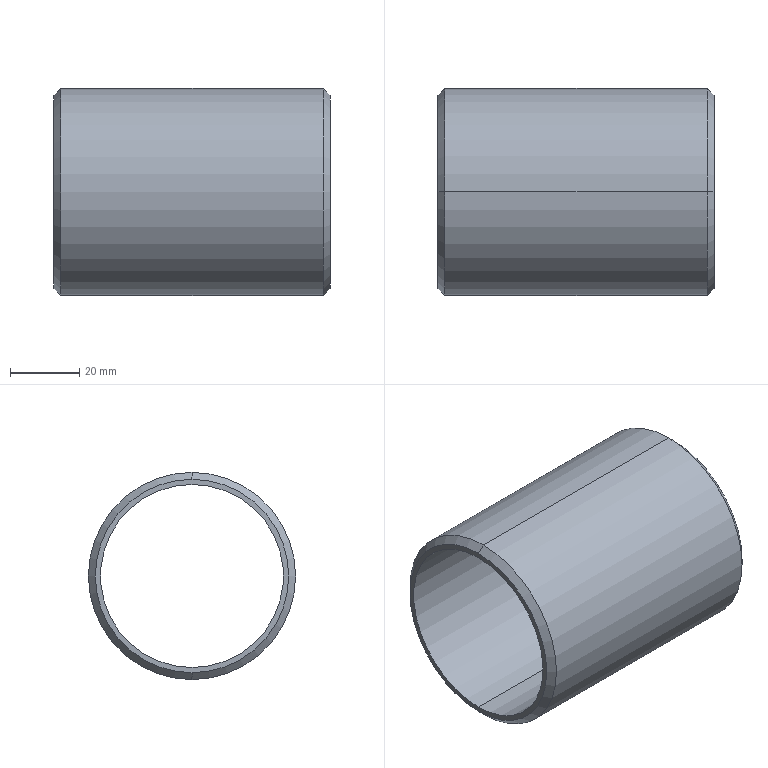Part | SolidWorks | features Chamfer 1, ExtruThin 1 | 1 solid | 10 faces | box 80 x 60 x 60 mm | volume 48963 mm3 | cone 4 | cylinder 4 | plane 2 | commonest cylinder face diameters 53 x2 60 x2
STEP:
#1=CARTESIAN_POINT('',(0.,0.,28.));
#2=VERTEX_POINT('',#1);
#3=CARTESIAN_POINT('',(0.,0.,-28.));
#4=VERTEX_POINT('',#3);
#5=CARTESIAN_POINT('',(0.,0.,0.));
#6=DIRECTION('',(-1.,0.,0.));
#7=DIRECTION('',(0.,0.,-1.));
#8=AXIS2_PLACEMENT_3D('',#5,#6,#7);
#9=CIRCLE('',#8,28.);
#10=EDGE_CURVE('',#2,#4,#9,.T.);
#11=ORIENTED_EDGE('',*,*,#10,.F.);
#12=CARTESIAN_POINT('',(2.,0.,30.));
#13=VERTEX_POINT('',#12);
#14=CARTESIAN_POINT('',(2.,0.,30.));
#15=DIRECTION('',(0.7071,0.,0.7071));
#16=VECTOR('',#15,1000.);
#17=LINE('',#14,#16);
#18=EDGE_CURVE('',#2,#13,#17,.T.);
#19=ORIENTED_EDGE('',*,*,#18,.T.);
#20=CARTESIAN_POINT('',(2.,0.,-30.));
#21=VERTEX_POINT('',#20);
#22=CARTESIAN_POINT('',(2.,0.,0.));
#23=DIRECTION('',(1.,0.,0.));
#24=DIRECTION('',(0.,0.,-1.));
#25=AXIS2_PLACEMENT_3D('',#22,#23,#24);
#26=CIRCLE('',#25,30.);
#27=EDGE_CURVE('',#21,#13,#26,.T.);
#28=ORIENTED_EDGE('',*,*,#27,.F.);
#29=CARTESIAN_POINT('',(2.,0.,-30.));
#30=DIRECTION('',(0.7071,0.,-0.7071));
#31=VECTOR('',#30,1000.);
#32=LINE('',#29,#31);
#33=EDGE_CURVE('',#4,#21,#32,.T.);
#34=ORIENTED_EDGE('',*,*,#33,.F.);
#35=EDGE_LOOP('',(#11,#19,#28,#34));
#36=FACE_OUTER_BOUND('',#35,.T.);
#37=CARTESIAN_POINT('',(2.,0.,0.));
#38=DIRECTION('',(1.,0.,0.));
#39=DIRECTION('',(0.,0.,-1.));
#40=AXIS2_PLACEMENT_3D('',#37,#38,#39);
#41=CONICAL_SURFACE('',#40,30.,0.7854);
#42=ADVANCED_FACE('',(#36),#41,.T.);
#43=CARTESIAN_POINT('',(80.,0.,-28.));
#44=VERTEX_POINT('',#43);
#45=CARTESIAN_POINT('',(80.,0.,28.));
#46=VERTEX_POINT('',#45);
#47=CARTESIAN_POINT('',(80.,0.,0.));
#48=DIRECTION('',(1.,0.,0.));
#49=DIRECTION('',(0.,0.,-1.));
#50=AXIS2_PLACEMENT_3D('',#47,#48,#49);
#51=CIRCLE('',#50,28.);
#52=EDGE_CURVE('',#44,#46,#51,.T.);
#53=ORIENTED_EDGE('',*,*,#52,.F.);
#54=CARTESIAN_POINT('',(78.,0.,-30.));
#55=VERTEX_POINT('',#54);
#56=CARTESIAN_POINT('',(80.,0.,-28.));
#57=DIRECTION('',(-0.7071,0.,-0.7071));
#58=VECTOR('',#57,1000.);
#59=LINE('',#56,#58);
#60=EDGE_CURVE('',#44,#55,#59,.T.);
#61=ORIENTED_EDGE('',*,*,#60,.T.);
#62=CARTESIAN_POINT('',(78.,0.,30.));
#63=VERTEX_POINT('',#62);
#64=CARTESIAN_POINT('',(78.,0.,0.));
#65=DIRECTION('',(-1.,0.,0.));
#66=DIRECTION('',(0.,0.,-1.));
#67=AXIS2_PLACEMENT_3D('',#64,#65,#66);
#68=CIRCLE('',#67,30.);
#69=EDGE_CURVE('',#63,#55,#68,.T.);
#70=ORIENTED_EDGE('',*,*,#69,.F.);
#71=CARTESIAN_POINT('',(80.,0.,28.));
#72=DIRECTION('',(-0.7071,0.,0.7071));
#73=VECTOR('',#72,1000.);
#74=LINE('',#71,#73);
#75=EDGE_CURVE('',#46,#63,#74,.T.);
#76=ORIENTED_EDGE('',*,*,#75,.F.);
#77=EDGE_LOOP('',(#53,#61,#70,#76));
#78=FACE_OUTER_BOUND('',#77,.T.);
#79=CARTESIAN_POINT('',(80.,0.,0.));
#80=DIRECTION('',(-1.,0.,0.));
#81=DIRECTION('',(0.,0.,1.));
#82=AXIS2_PLACEMENT_3D('',#79,#80,#81);
#83=CONICAL_SURFACE('',#82,28.,0.7854);
#84=ADVANCED_FACE('',(#78),#83,.T.);
#85=CARTESIAN_POINT('',(80.,0.,26.5));
#86=VERTEX_POINT('',#85);
#87=CARTESIAN_POINT('',(80.,0.,-26.5));
#88=VERTEX_POINT('',#87);
#89=CARTESIAN_POINT('',(80.,0.,0.));
#90=DIRECTION('',(1.,0.,0.));
#91=DIRECTION('',(0.,0.,-1.));
#92=AXIS2_PLACEMENT_3D('',#89,#90,#91);
#93=CIRCLE('',#92,26.5);
#94=EDGE_CURVE('',#86,#88,#93,.T.);
#95=ORIENTED_EDGE('',*,*,#94,.T.);
#96=CARTESIAN_POINT('',(0.,0.,-26.5));
#97=VERTEX_POINT('',#96);
#98=CARTESIAN_POINT('',(80.,0.,-26.5));
#99=DIRECTION('',(-1.,0.,0.));
#100=VECTOR('',#99,1000.);
#101=LINE('',#98,#100);
#102=EDGE_CURVE('',#88,#97,#101,.T.);
#103=ORIENTED_EDGE('',*,*,#102,.T.);
#104=CARTESIAN_POINT('',(0.,0.,26.5));
#105=VERTEX_POINT('',#104);
#106=CARTESIAN_POINT('',(0.,0.,0.));
#107=DIRECTION('',(1.,0.,0.));
#108=DIRECTION('',(0.,0.,-1.));
#109=AXIS2_PLACEMENT_3D('',#106,#107,#108);
#110=CIRCLE('',#109,26.5);
#111=EDGE_CURVE('',#105,#97,#110,.T.);
#112=ORIENTED_EDGE('',*,*,#111,.F.);
#113=CARTESIAN_POINT('',(80.,0.,26.5));
#114=DIRECTION('',(-1.,0.,0.));
#115=VECTOR('',#114,1000.);
#116=LINE('',#113,#115);
#117=EDGE_CURVE('',#86,#105,#116,.T.);
#118=ORIENTED_EDGE('',*,*,#117,.F.);
#119=EDGE_LOOP('',(#95,#103,#112,#118));
#120=FACE_OUTER_BOUND('',#119,.T.);
#121=CARTESIAN_POINT('',(80.,0.,0.));
#122=DIRECTION('',(-1.,0.,0.));
#123=DIRECTION('',(0.,0.,1.));
#124=AXIS2_PLACEMENT_3D('',#121,#122,#123);
#125=CYLINDRICAL_SURFACE('',#124,26.5);
#126=ADVANCED_FACE('',(#120),#125,.F.);
#127=ORIENTED_EDGE('',*,*,#69,.T.);
#128=CARTESIAN_POINT('',(80.,0.,-30.));
#129=DIRECTION('',(-1.,0.,0.));
#130=VECTOR('',#129,1000.);
#131=LINE('',#128,#130);
#132=EDGE_CURVE('',#55,#21,#131,.T.);
#133=ORIENTED_EDGE('',*,*,#132,.T.);
#134=ORIENTED_EDGE('',*,*,#27,.T.);
#135=CARTESIAN_POINT('',(80.,0.,30.));
#136=DIRECTION('',(-1.,0.,0.));
#137=VECTOR('',#136,1000.);
#138=LINE('',#135,#137);
#139=EDGE_CURVE('',#63,#13,#138,.T.);
#140=ORIENTED_EDGE('',*,*,#139,.F.);
#141=EDGE_LOOP('',(#127,#133,#134,#140));
#142=FACE_OUTER_BOUND('',#141,.T.);
#143=CARTESIAN_POINT('',(80.,0.,0.));
#144=DIRECTION('',(-1.,0.,0.));
#145=DIRECTION('',(0.,0.,1.));
#146=AXIS2_PLACEMENT_3D('',#143,#144,#145);
#147=CYLINDRICAL_SURFACE('',#146,30.);
#148=ADVANCED_FACE('',(#142),#147,.T.);
#149=CARTESIAN_POINT('',(80.,0.,0.));
#150=DIRECTION('',(1.,0.,0.));
#151=DIRECTION('',(0.,0.,-1.));
#152=AXIS2_PLACEMENT_3D('',#149,#150,#151);
#153=CIRCLE('',#152,28.);
#154=EDGE_CURVE('',#46,#44,#153,.T.);
#155=ORIENTED_EDGE('',*,*,#154,.T.);
#156=ORIENTED_EDGE('',*,*,#52,.T.);
#157=EDGE_LOOP('',(#155,#156));
#158=FACE_OUTER_BOUND('',#157,.T.);
#159=ORIENTED_EDGE('',*,*,#94,.F.);
#160=CARTESIAN_POINT('',(80.,0.,0.));
#161=DIRECTION('',(1.,0.,0.));
#162=DIRECTION('',(0.,0.,-1.));
#163=AXIS2_PLACEMENT_3D('',#160,#161,#162);
#164=CIRCLE('',#163,26.5);
#165=EDGE_CURVE('',#88,#86,#164,.T.);
#166=ORIENTED_EDGE('',*,*,#165,.F.);
#167=EDGE_LOOP('',(#159,#166));
#168=FACE_BOUND('',#167,.T.);
#169=CARTESIAN_POINT('',(80.,0.,0.));
#170=DIRECTION('',(1.,0.,0.));
#171=DIRECTION('',(0.,0.,-1.));
#172=AXIS2_PLACEMENT_3D('',#169,#170,#171);
#173=PLANE('',#172);
#174=ADVANCED_FACE('',(#158,#168),#173,.T.);
#175=CARTESIAN_POINT('',(0.,0.,0.));
#176=DIRECTION('',(-1.,0.,0.));
#177=DIRECTION('',(0.,0.,-1.));
#178=AXIS2_PLACEMENT_3D('',#175,#176,#177);
#179=CIRCLE('',#178,28.);
#180=EDGE_CURVE('',#4,#2,#179,.T.);
#181=ORIENTED_EDGE('',*,*,#180,.T.);
#182=ORIENTED_EDGE('',*,*,#10,.T.);
#183=EDGE_LOOP('',(#181,#182));
#184=FACE_OUTER_BOUND('',#183,.T.);
#185=ORIENTED_EDGE('',*,*,#111,.T.);
#186=CARTESIAN_POINT('',(0.,0.,0.));
#187=DIRECTION('',(1.,0.,0.));
#188=DIRECTION('',(0.,0.,-1.));
#189=AXIS2_PLACEMENT_3D('',#186,#187,#188);
#190=CIRCLE('',#189,26.5);
#191=EDGE_CURVE('',#97,#105,#190,.T.);
#192=ORIENTED_EDGE('',*,*,#191,.T.);
#193=EDGE_LOOP('',(#185,#192));
#194=FACE_BOUND('',#193,.T.);
#195=CARTESIAN_POINT('',(0.,0.,0.));
#196=DIRECTION('',(1.,0.,0.));
#197=DIRECTION('',(0.,0.,-1.));
#198=AXIS2_PLACEMENT_3D('',#195,#196,#197);
#199=PLANE('',#198);
#200=ADVANCED_FACE('',(#184,#194),#199,.F.);
#201=ORIENTED_EDGE('',*,*,#132,.F.);
#202=CARTESIAN_POINT('',(78.,0.,0.));
#203=DIRECTION('',(-1.,0.,0.));
#204=DIRECTION('',(0.,0.,-1.));
#205=AXIS2_PLACEMENT_3D('',#202,#203,#204);
#206=CIRCLE('',#205,30.);
#207=EDGE_CURVE('',#55,#63,#206,.T.);
#208=ORIENTED_EDGE('',*,*,#207,.T.);
#209=ORIENTED_EDGE('',*,*,#139,.T.);
#210=CARTESIAN_POINT('',(2.,0.,0.));
#211=DIRECTION('',(1.,0.,0.));
#212=DIRECTION('',(0.,0.,-1.));
#213=AXIS2_PLACEMENT_3D('',#210,#211,#212);
#214=CIRCLE('',#213,30.);
#215=EDGE_CURVE('',#13,#21,#214,.T.);
#216=ORIENTED_EDGE('',*,*,#215,.T.);
#217=EDGE_LOOP('',(#201,#208,#209,#216));
#218=FACE_OUTER_BOUND('',#217,.T.);
#219=CARTESIAN_POINT('',(80.,0.,0.));
#220=DIRECTION('',(-1.,0.,0.));
#221=DIRECTION('',(0.,0.,1.));
#222=AXIS2_PLACEMENT_3D('',#219,#220,#221);
#223=CYLINDRICAL_SURFACE('',#222,30.);
#224=ADVANCED_FACE('',(#218),#223,.T.);
#225=ORIENTED_EDGE('',*,*,#102,.F.);
#226=ORIENTED_EDGE('',*,*,#165,.T.);
#227=ORIENTED_EDGE('',*,*,#117,.T.);
#228=ORIENTED_EDGE('',*,*,#191,.F.);
#229=EDGE_LOOP('',(#225,#226,#227,#228));
#230=FACE_OUTER_BOUND('',#229,.T.);
#231=CARTESIAN_POINT('',(80.,0.,0.));
#232=DIRECTION('',(-1.,0.,0.));
#233=DIRECTION('',(0.,0.,1.));
#234=AXIS2_PLACEMENT_3D('',#231,#232,#233);
#235=CYLINDRICAL_SURFACE('',#234,26.5);
#236=ADVANCED_FACE('',(#230),#235,.F.);
#237=ORIENTED_EDGE('',*,*,#60,.F.);
#238=ORIENTED_EDGE('',*,*,#154,.F.);
#239=ORIENTED_EDGE('',*,*,#75,.T.);
#240=ORIENTED_EDGE('',*,*,#207,.F.);
#241=EDGE_LOOP('',(#237,#238,#239,#240));
#242=FACE_OUTER_BOUND('',#241,.T.);
#243=CARTESIAN_POINT('',(80.,0.,0.));
#244=DIRECTION('',(-1.,0.,0.));
#245=DIRECTION('',(0.,0.,1.));
#246=AXIS2_PLACEMENT_3D('',#243,#244,#245);
#247=CONICAL_SURFACE('',#246,28.,0.7854);
#248=ADVANCED_FACE('',(#242),#247,.T.);
#249=ORIENTED_EDGE('',*,*,#18,.F.);
#250=ORIENTED_EDGE('',*,*,#180,.F.);
#251=ORIENTED_EDGE('',*,*,#33,.T.);
#252=ORIENTED_EDGE('',*,*,#215,.F.);
#253=EDGE_LOOP('',(#249,#250,#251,#252));
#254=FACE_OUTER_BOUND('',#253,.T.);
#255=CARTESIAN_POINT('',(2.,0.,0.));
#256=DIRECTION('',(1.,0.,0.));
#257=DIRECTION('',(0.,0.,-1.));
#258=AXIS2_PLACEMENT_3D('',#255,#256,#257);
#259=CONICAL_SURFACE('',#258,30.,0.7854);
#260=ADVANCED_FACE('',(#254),#259,.T.);
#261=CLOSED_SHELL('',(#42,#84,#126,#148,#174,#200,#224,#236,#248,#260));
#262=MANIFOLD_SOLID_BREP('',#261);
#263=CARTESIAN_POINT('',(0.,0.,0.));
#264=DIRECTION('',(0.,0.,1.));
#265=DIRECTION('',(1.,0.,0.));
#266=AXIS2_PLACEMENT_3D('',#263,#264,#265);
#267=(LENGTH_UNIT()NAMED_UNIT(*)SI_UNIT(.MILLI.,.METRE.));
#268=UNCERTAINTY_MEASURE_WITH_UNIT(LENGTH_MEASURE(0.00001),#267,'','');
#269=(NAMED_UNIT(*)PLANE_ANGLE_UNIT()SI_UNIT($,.RADIAN.));
#270=(NAMED_UNIT(*)SI_UNIT($,.STERADIAN.)SOLID_ANGLE_UNIT());
#271=(GEOMETRIC_REPRESENTATION_CONTEXT(3)GLOBAL_UNCERTAINTY_ASSIGNED_CONTEXT((#268))GLOBAL_UNIT_ASSIGNED_CONTEXT((#267,#269,#270))REPRESENTATION_CONTEXT('',''));
#272=ADVANCED_BREP_SHAPE_REPRESENTATION('',(#262,#266),#271);